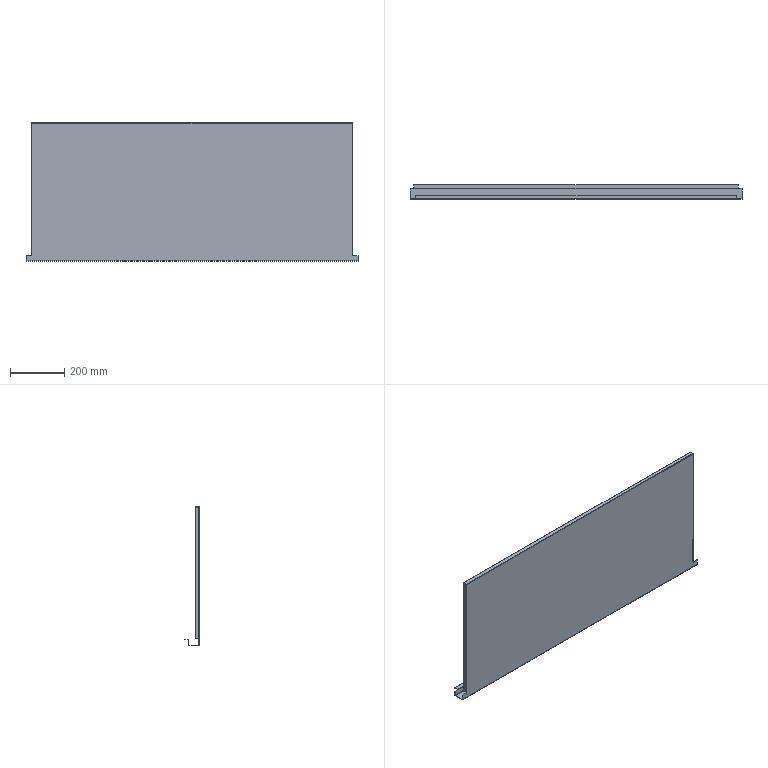Part | SolidWorks | features EdgeFlange 4, ICE 2, FlatPattern 1, SMBaseFlange 1, SheetMetal 1 | 1 solid | 66 faces | box 1220 x 53.8 x 510 mm | volume 861259 mm3 | plane 50 | cylinder 12 | spline 4 | commonest cylinder face diameters 0.9 x6 3.3 x6